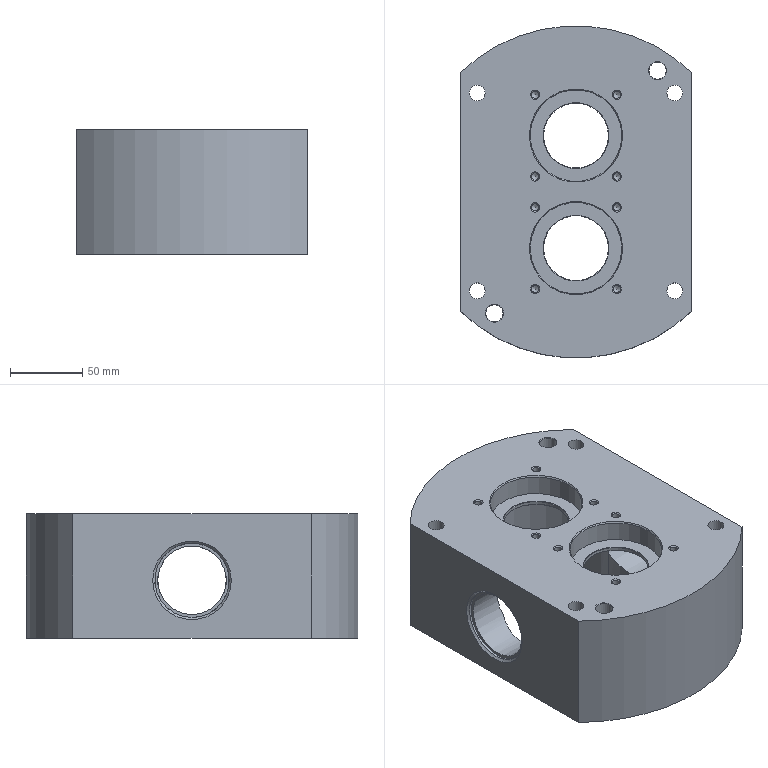NC program | NX | posted with a generic post | part box 160 x 230 x 86 mm
Lines 1 to 85 of 2142:
N10 G17 G21 G94 G90
(DRILLING , TOOL : ZXZ)
N12 T01 M6
N14 G54
N16 G17 G0 G90 X-68.5 Y-68.5 B0. C0. S5000 M3
N18 G43 Z30. H1
N20 G94 G81 G98 Z-1. F250. R3.
N22 X-67.284 Y-28.284
N24 X-39. Y0.
N26 X-10.716 Y-28.284
N28 X10.716
N30 X68.5 Y-68.5
N32 X84. Y-56.5
N34 X67.284 Y-28.284
N36 X39. Y0.
N38 X67.284 Y28.284
N40 X68.5 Y68.5
N42 X10.716 Y28.284
N44 X-10.716
N46 X-67.284
N48 X-84. Y56.5
N50 X-68.5 Y68.5
N52 G80
N54 G0 X-68.5 Y68.5 Z30.
N56 M5
(DRILLING_COPY , TOOL : 11.0ZT)
N58 T09 M6
N60 G54
N62 G17 G0 G90 X68.5 Y-68.5 B0. C0. S2000 M3
N64 G43 Z30. H9
N66 G94 G83 G98 Z-91.305 F150. Q2. R3.
N68 X-68.5
N70 Y68.5
N72 X68.5
N74 G80
N76 G0 X68.5 Y68.5 Z30.
N78 M5
(DRILLING_COPY_COPY , TOOL : 11.8ZT)
N80 T08 M6
N82 G54
N84 G17 G0 G90 X84. Y-56.5 B0. C0. S2000 M3
N86 G43 Z30. H8
N88 G94 G83 G98 Z-91.045 F150. Q2. R3.
N90 X-84. Y56.5
N92 G80
N94 G0 X-84. Y56.5 Z30.
N96 M5
(DRILLING_COPY_COPY_COPY , TOOL : 12.0JD)
N98 T18 M6
N100 G54
N102 G17 G0 G90 X84. Y-56.5 B0. C0. S800 M3
N104 G43 Z30. H18
N106 G94 G85 G98 Z-86.5 F40. R3.
N108 X-84. Y56.5
N110 G80
N112 G0 X-84. Y56.5 Z30.
N114 M5
(DRILLING_COPY_COPY_1 , TOOL : 5.0ZT)
N116 T15 M6
N118 G54
N120 G17 G0 G90 X67.284 Y-28.284 B0. C0. S2000 M3
N122 G43 Z30. H15
N124 G94 G83 G98 Z-14.502 F150. Q2. R3.
N126 Y28.284
N128 X10.716
N130 X-10.716
N132 X-67.284
N134 Y-28.284
N136 X-10.716
N138 X10.716
N140 G80
N142 G0 X10.716 Y-28.284 Z30.
N144 M5